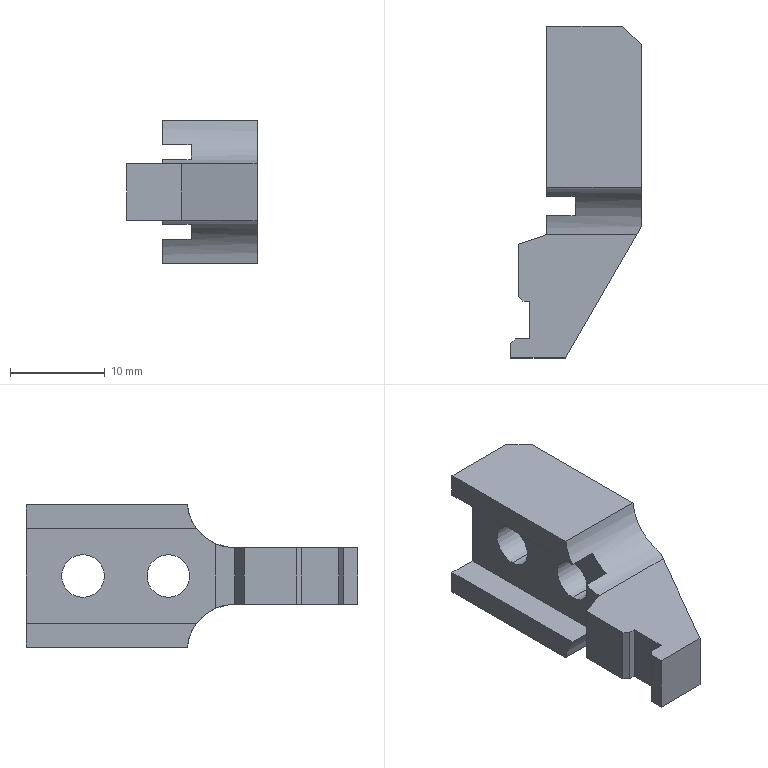Part | STEP file | PN_0004 | 1 solid | 30 faces | box 13.8 x 35 x 15 mm | volume 2765 mm3 | plane 24 | cylinder 6 | commonest cylinder face diameters 4.5 x4 10 x2